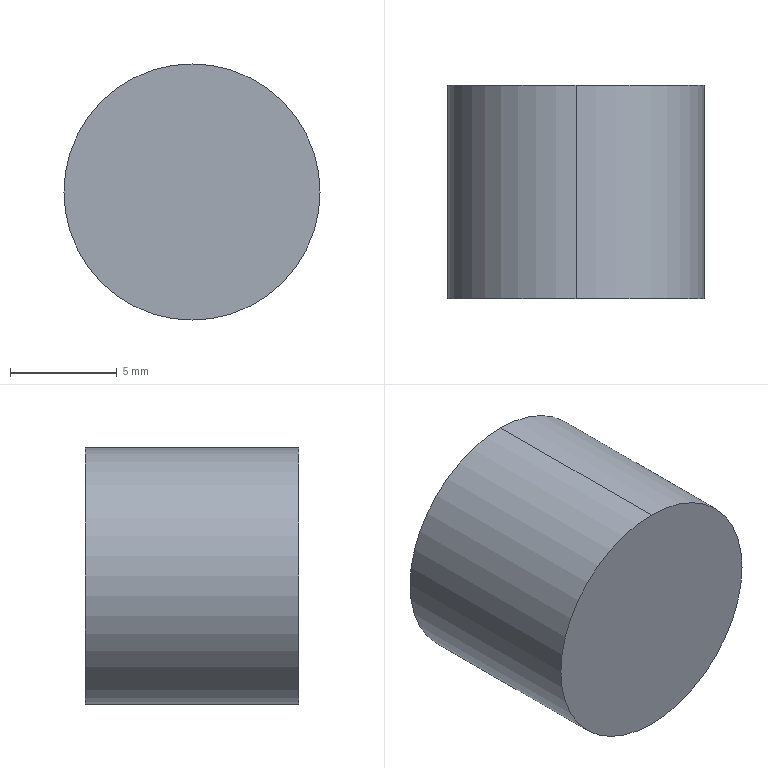Part | SolidWorks | features BaseBody 1 | 1 solid | 4 faces | box 12 x 10 x 12 mm | volume 1131 mm3 | cylinder 2 | plane 2 | commonest cylinder face diameters 12 x2
STEP:
#1=CARTESIAN_POINT('',(-31.,274.5,62.));
#2=VERTEX_POINT('',#1);
#3=CARTESIAN_POINT('',(-31.,274.5,50.));
#4=VERTEX_POINT('',#3);
#5=CARTESIAN_POINT('',(-31.,274.5,56.));
#6=DIRECTION('',(0.,1.,0.));
#7=DIRECTION('',(0.,0.,1.));
#8=AXIS2_PLACEMENT_3D('',#5,#6,#7);
#9=CIRCLE('',#8,6.);
#10=EDGE_CURVE('',#2,#4,#9,.T.);
#11=ORIENTED_EDGE('',*,*,#10,.T.);
#12=CARTESIAN_POINT('',(-31.,284.5,50.));
#13=VERTEX_POINT('',#12);
#14=CARTESIAN_POINT('',(-31.,274.5,50.));
#15=DIRECTION('',(0.,1.,0.));
#16=VECTOR('',#15,1000.);
#17=LINE('',#14,#16);
#18=EDGE_CURVE('',#4,#13,#17,.T.);
#19=ORIENTED_EDGE('',*,*,#18,.T.);
#20=CARTESIAN_POINT('',(-31.,284.5,62.));
#21=VERTEX_POINT('',#20);
#22=CARTESIAN_POINT('',(-31.,284.5,56.));
#23=DIRECTION('',(0.,-1.,0.));
#24=DIRECTION('',(0.,0.,1.));
#25=AXIS2_PLACEMENT_3D('',#22,#23,#24);
#26=CIRCLE('',#25,6.);
#27=EDGE_CURVE('',#13,#21,#26,.T.);
#28=ORIENTED_EDGE('',*,*,#27,.T.);
#29=CARTESIAN_POINT('',(-31.,274.5,62.));
#30=DIRECTION('',(0.,1.,0.));
#31=VECTOR('',#30,1000.);
#32=LINE('',#29,#31);
#33=EDGE_CURVE('',#2,#21,#32,.T.);
#34=ORIENTED_EDGE('',*,*,#33,.F.);
#35=EDGE_LOOP('',(#11,#19,#28,#34));
#36=FACE_OUTER_BOUND('',#35,.T.);
#37=CARTESIAN_POINT('',(-31.,274.5,56.));
#38=DIRECTION('',(0.,1.,0.));
#39=DIRECTION('',(0.,0.,1.));
#40=AXIS2_PLACEMENT_3D('',#37,#38,#39);
#41=CYLINDRICAL_SURFACE('',#40,6.);
#42=ADVANCED_FACE('',(#36),#41,.T.);
#43=ORIENTED_EDGE('',*,*,#18,.F.);
#44=CARTESIAN_POINT('',(-31.,274.5,56.));
#45=DIRECTION('',(0.,1.,0.));
#46=DIRECTION('',(0.,0.,1.));
#47=AXIS2_PLACEMENT_3D('',#44,#45,#46);
#48=CIRCLE('',#47,6.);
#49=EDGE_CURVE('',#4,#2,#48,.T.);
#50=ORIENTED_EDGE('',*,*,#49,.T.);
#51=ORIENTED_EDGE('',*,*,#33,.T.);
#52=CARTESIAN_POINT('',(-31.,284.5,56.));
#53=DIRECTION('',(0.,-1.,0.));
#54=DIRECTION('',(0.,0.,1.));
#55=AXIS2_PLACEMENT_3D('',#52,#53,#54);
#56=CIRCLE('',#55,6.);
#57=EDGE_CURVE('',#21,#13,#56,.T.);
#58=ORIENTED_EDGE('',*,*,#57,.T.);
#59=EDGE_LOOP('',(#43,#50,#51,#58));
#60=FACE_OUTER_BOUND('',#59,.T.);
#61=CARTESIAN_POINT('',(-31.,274.5,56.));
#62=DIRECTION('',(0.,1.,0.));
#63=DIRECTION('',(0.,0.,1.));
#64=AXIS2_PLACEMENT_3D('',#61,#62,#63);
#65=CYLINDRICAL_SURFACE('',#64,6.);
#66=ADVANCED_FACE('',(#60),#65,.T.);
#67=ORIENTED_EDGE('',*,*,#10,.F.);
#68=ORIENTED_EDGE('',*,*,#49,.F.);
#69=EDGE_LOOP('',(#67,#68));
#70=FACE_OUTER_BOUND('',#69,.T.);
#71=CARTESIAN_POINT('',(-31.,274.5,56.));
#72=DIRECTION('',(0.,1.,0.));
#73=DIRECTION('',(0.,0.,1.));
#74=AXIS2_PLACEMENT_3D('',#71,#72,#73);
#75=PLANE('',#74);
#76=ADVANCED_FACE('',(#70),#75,.F.);
#77=ORIENTED_EDGE('',*,*,#57,.F.);
#78=ORIENTED_EDGE('',*,*,#27,.F.);
#79=EDGE_LOOP('',(#77,#78));
#80=FACE_OUTER_BOUND('',#79,.T.);
#81=CARTESIAN_POINT('',(-31.,284.5,56.));
#82=DIRECTION('',(0.,1.,0.));
#83=DIRECTION('',(0.,0.,1.));
#84=AXIS2_PLACEMENT_3D('',#81,#82,#83);
#85=PLANE('',#84);
#86=ADVANCED_FACE('',(#80),#85,.T.);
#87=CLOSED_SHELL('',(#42,#66,#76,#86));
#88=MANIFOLD_SOLID_BREP('',#87);
#89=CARTESIAN_POINT('',(0.,0.,0.));
#90=DIRECTION('',(0.,0.,1.));
#91=DIRECTION('',(1.,0.,0.));
#92=AXIS2_PLACEMENT_3D('',#89,#90,#91);
#93=(LENGTH_UNIT()NAMED_UNIT(*)SI_UNIT(.MILLI.,.METRE.));
#94=UNCERTAINTY_MEASURE_WITH_UNIT(LENGTH_MEASURE(0.00001),#93,'','');
#95=(NAMED_UNIT(*)PLANE_ANGLE_UNIT()SI_UNIT($,.RADIAN.));
#96=(NAMED_UNIT(*)SI_UNIT($,.STERADIAN.)SOLID_ANGLE_UNIT());
#97=(GEOMETRIC_REPRESENTATION_CONTEXT(3)GLOBAL_UNCERTAINTY_ASSIGNED_CONTEXT((#94))GLOBAL_UNIT_ASSIGNED_CONTEXT((#93,#95,#96))REPRESENTATION_CONTEXT('',''));
#98=ADVANCED_BREP_SHAPE_REPRESENTATION('',(#88,#92),#97);